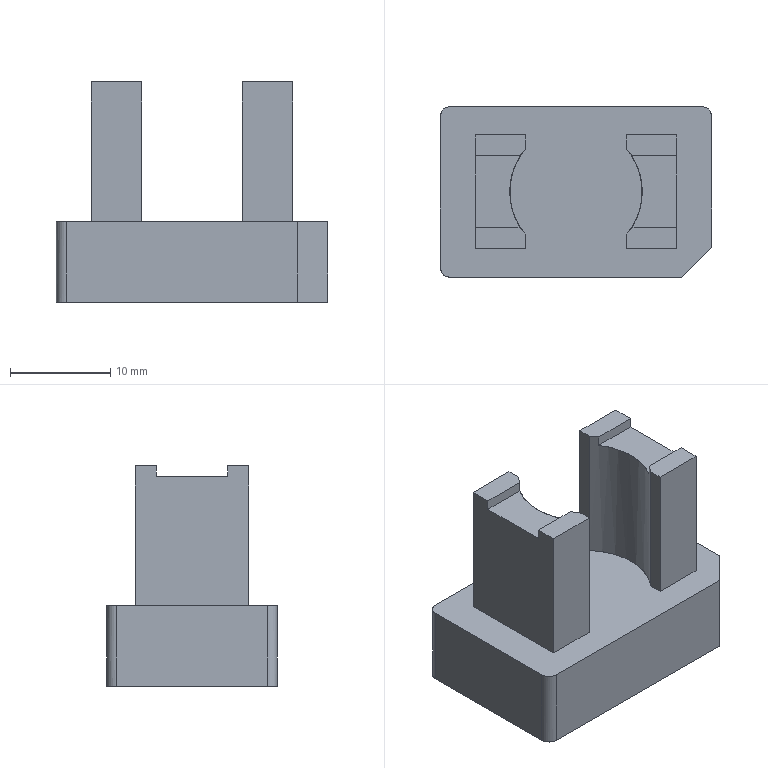NC program | PowerMill | posted with a generic post | part box 27 x 17 x 21.929 mm
Lines 5206 to 6181 of 116051:
N5303 M6
N5304 S18000 M03
N5305 G00 G90 X0.0 Y0.0
N5306 G43 Z9.7986 H2
N5307
N5308 G05 P10000 R4
N5309 X-12.0223 Y7.7454
N5310 Z0.7937
N5311 G01 Z-0.4063 F3600.0
N5312 X-11.8798 Y7.5778 F6000.0
N5313 X-11.4537 Y7.0768
N5314 X-11.2252 Y7.2711
N5315 X-10.7372 Y7.5319
N5316 X-10.2491 Y7.6444
N5317 X-4.8805 Y7.6519
N5318 X-4.3936 Y7.5648
N5319 X-3.9044 Y7.3367
N5320 X-3.5801 Y7.0768
N5321 X-3.4164 Y6.8936
N5322 X-3.218 Y6.5887
N5323 X-3.0368 Y6.1007
N5324 X-2.9865 Y5.6126
N5325 X-2.9947 Y4.1484
N5326 X-3.1019 Y3.6604
N5327 X-3.3555 Y3.1723
N5328 X-4.1012 Y2.1962
N5329 X-4.3925 Y1.9412
N5330 X-4.8182 Y1.7082
N5331 X-5.3686 Y1.5753
N5332 X-5.8566 Y1.5663
N5333 X-9.7611
N5334 X-10.2491 Y1.5765
N5335 X-10.7372 Y1.6889
N5336 X-11.2252 Y1.9498
N5337 X-11.5046 Y2.1962
N5338 X-11.7133 Y2.4594
N5339 X-11.8424 Y2.6843
N5340 X-12.0083 Y3.1723
N5341 X-12.0474 Y3.6604
N5342 Y5.6126
N5343 X-11.997 Y6.1007
N5344 X-11.816 Y6.5887
N5345 X-11.7133 Y6.7615
N5346 X-11.4537 Y7.0768
N5347 X-11.8798 Y7.5778
N5348 G00 Z3.7937
N5349 G01 X11.7989 Y7.9457 F10000.0
N5350 G00 Z0.7937
N5351 G01 Z-0.4063 F3600.0
N5352 X11.6564 Y7.7781 F6000.0
N5353 X11.2252 Y7.2711
N5354 X11.4537 Y7.0768
N5355 X11.7133 Y6.7615
N5356 X11.816 Y6.5887
N5357 X11.997 Y6.1007
N5358 X12.0474 Y5.6126
N5359 Y3.6604
N5360 X12.0083 Y3.1723
N5361 X11.8425 Y2.6843
N5362 X11.7133 Y2.4594
N5363 X11.5046 Y2.1962
N5364 X11.2252 Y1.9498
N5365 X10.7875 Y1.7082
N5366 X10.2491 Y1.5765
N5367 X9.7611 Y1.5663
N5368 X5.8566
N5369 X5.3686 Y1.5753
N5370 X4.8805 Y1.6846
N5371 X4.3925 Y1.9412
N5372 X4.1012 Y2.1962
N5373 X3.3555 Y3.1723
N5374 X3.1019 Y3.6604
N5375 X2.9947 Y4.1484
N5376 X2.9865 Y5.6126
N5377 X3.0368 Y6.1007
N5378 X3.218 Y6.5887
N5379 X3.4164 Y6.8936
N5380 X3.5801 Y7.0768
N5381 X3.9044 Y7.3367
N5382 X4.3925 Y7.5644
N5383 X4.8805 Y7.6519
N5384 X9.7611 Y7.6547
N5385 X10.2491 Y7.6444
N5386 X10.6403 Y7.5648
N5387 X11.2252 Y7.2711
N5388 X11.6564 Y7.7781
N5389 G00 Z3.7937
N5390 G01 X12.0223 Y-7.7454 F10000.0
N5391 G00 Z0.7937
N5392 G01 Z-0.4063 F3600.0
N5393 X11.8798 Y-7.5778 F6000.0
N5394 X11.4537 Y-7.0768
N5395 X11.2252 Y-7.2711
N5396 X10.6403 Y-7.5648
N5397 X10.2491 Y-7.6444
N5398 X4.8805 Y-7.6519
N5399 X4.3936 Y-7.5648
N5400 X3.9044 Y-7.3367
N5401 X3.5801 Y-7.0768
N5402 X3.4164 Y-6.8936
N5403 X3.218 Y-6.5887
N5404 X3.0368 Y-6.1007
N5405 X2.9865 Y-5.6126
N5406 X2.9947 Y-4.1484
N5407 X3.1019 Y-3.6604
N5408 X3.3555 Y-3.1723
N5409 X4.0954 Y-2.1962
N5410 X4.3925 Y-1.9302
N5411 X4.7819 Y-1.7082
N5412 X5.3686 Y-1.5561
N5413 X5.8566 Y-1.5458
N5414 X9.7611
N5415 X10.2491 Y-1.556
N5416 X10.7372 Y-1.6684
N5417 X11.2252 Y-1.9294
N5418 X11.5235 Y-2.1962
N5419 X11.7133 Y-2.4389
N5420 X11.8524 Y-2.6843
N5421 X12.0123 Y-3.1723
N5422 X12.0474 Y-3.6604
N5423 Y-5.6126
N5424 X11.997 Y-6.1007
N5425 X11.816 Y-6.5887
N5426 X11.7133 Y-6.7615
N5427 X11.4537 Y-7.0768
N5428 X11.8798 Y-7.5778
N5429 G00 Z3.7937
N5430 G01 X-11.7989 Y-7.9457 F10000.0
N5431 G00 Z0.7937
N5432 G01 Z-0.4063 F3600.0
N5433 X-11.6564 Y-7.7781 F6000.0
N5434 X-11.2252 Y-7.2711
N5435 X-11.4537 Y-7.0768
N5436 X-11.7133 Y-6.7615
N5437 X-11.816 Y-6.5887
N5438 X-11.997 Y-6.1007
N5439 X-12.0474 Y-5.6126
N5440 Y-3.6604
N5441 X-12.0122 Y-3.1723
N5442 X-11.8524 Y-2.6843
N5443 X-11.7133 Y-2.4389
N5444 X-11.5235 Y-2.1962
N5445 X-11.2252 Y-1.9294
N5446 X-10.8369 Y-1.7082
N5447 X-10.2491 Y-1.556
N5448 X-9.7611 Y-1.5458
N5449 X-5.8566
N5450 X-5.3686 Y-1.5561
N5451 X-4.8805 Y-1.6689
N5452 X-4.3925 Y-1.9302
N5453 X-4.0953 Y-2.1962
N5454 X-3.6415 Y-2.795
N5455 X-2.1015 Y-1.6849
N5456 X-0.5876 Y-0.5937
N5457 G03 X-0.1383 Y-0.87 I0.5563 J0.401
N5458 G03 X0.6469 Y-0.2942 I0.107 J0.6773
N5459 G01 X0.7056 Y0.0984
N5460 G03 X-0.6425 Y0.3114 I-0.675 J0.1009
N5461 G01 X-0.7077 Y-0.0801
N5462 G03 X-0.5876 Y-0.5937 I0.6764 J-0.1126
N5463 G01 X-2.1015 Y-1.6849
N5464 X-2.2353 Y-1.516
N5465 X-2.3761 Y-1.3529
N5466 X-2.7155 Y-0.9761
N5467 X-3.2416 Y-0.4349
N5468 G02 X-3.2218 Y0.4642 I0.4476 J0.4399
N5469 G01 X-2.7107 Y0.9402
N5470 G03 X-1.446 Y2.647 I-3.9757 J4.2682
N5471 G01 X-1.1868 Y3.1772
N5472 G02 X-0.4686 Y3.6259 I0.7188 J-0.3513
N5473 G01 X0.4658 Y3.6266
N5474 G02 X1.1573 Y3.2298 I0.0005 J-0.8
N5475 G01 X1.7618 Y2.1941
N5476 X2.0603 Y1.7401
N5477 X2.4055 Y1.3206
N5478 X2.7297 Y0.9668
N5479 X3.2386 Y0.4462
N5480 G02 X3.2213 Y-0.4564 I-0.4498 J-0.4428
N5481 G01 X2.7083 Y-0.939
N5482 G03 X1.3418 Y-2.8419 I4.1817 J-4.445
N5483 G01 X1.1966 Y-3.1588
N5484 G02 X0.4702 Y-3.6256 I-0.7273 J0.3332
N5485 G01 X-0.4653 Y-3.6267
N5486 G02 X-1.1572 Y-3.23 I-0.001 J0.8
N5487 G01 X-1.7618 Y-2.1941
N5488 X-1.924 Y-1.9344
N5489 X-2.1015 Y-1.6849
N5490 X-3.6415 Y-2.795
N5491 X-3.3555 Y-3.1723
N5492 X-3.1019 Y-3.6604
N5493 X-2.9947 Y-4.1484
N5494 X-2.9865 Y-5.6126
N5495 X-3.0368 Y-6.1007
N5496 X-3.218 Y-6.5887
N5497 X-3.4164 Y-6.8936
N5498 X-3.5801 Y-7.0768
N5499 X-3.9044 Y-7.3367
N5500 X-4.3936 Y-7.5648
N5501 X-4.8805 Y-7.6519
N5502 X-9.7611 Y-7.6547
N5503 X-10.2491 Y-7.6444
N5504 X-10.6403 Y-7.5648
N5505 X-11.2252 Y-7.2711
N5506 X-11.6564 Y-7.7781
N5507 G00 Z3.5984
N5508 G01 X-12.0223 Y7.7454 F10000.0
N5509 G00 Z0.5985
N5510 G01 Z-0.6015 F3600.0
N5511 X-11.8798 Y7.5778 F6000.0
N5512 X-11.4537 Y7.0768
N5513 X-11.2252 Y7.2711
N5514 X-10.7372 Y7.5319
N5515 X-10.2491 Y7.6444
N5516 X-4.8805 Y7.6519
N5517 X-4.3936 Y7.5648
N5518 X-3.9044 Y7.3367
N5519 X-3.5801 Y7.0768
N5520 X-3.4164 Y6.8936
N5521 X-3.218 Y6.5887
N5522 X-3.0368 Y6.1007
N5523 X-2.9865 Y5.6126
N5524 X-2.9947 Y4.1484
N5525 X-3.1019 Y3.6604
N5526 X-3.3555 Y3.1723
N5527 X-4.1012 Y2.1962
N5528 X-4.3925 Y1.9411
N5529 X-4.8182 Y1.7082
N5530 X-5.3686 Y1.5753
N5531 X-5.8566 Y1.5663
N5532 X-9.7611
N5533 X-10.2491 Y1.5764
N5534 X-10.7372 Y1.6889
N5535 X-11.2252 Y1.9497
N5536 X-11.5046 Y2.1962
N5537 X-11.7133 Y2.4593
N5538 X-11.8425 Y2.6843
N5539 X-12.0083 Y3.1723
N5540 X-12.0474 Y3.6604
N5541 Y5.6126
N5542 X-11.997 Y6.1007
N5543 X-11.816 Y6.5887
N5544 X-11.7133 Y6.7615
N5545 X-11.4537 Y7.0768
N5546 X-11.8798 Y7.5778
N5547 G00 Z3.5984
N5548 G01 X11.7989 Y7.9457 F10000.0
N5549 G00 Z0.5985
N5550 G01 Z-0.6015 F3600.0
N5551 X11.6564 Y7.7781 F6000.0
N5552 X11.2252 Y7.2711
N5553 X11.4537 Y7.0768
N5554 X11.7133 Y6.7615
N5555 X11.816 Y6.5887
N5556 X11.997 Y6.1007
N5557 X12.0474 Y5.6126
N5558 Y3.6604
N5559 X12.0083 Y3.1723
N5560 X11.8425 Y2.6843
N5561 X11.7133 Y2.4593
N5562 X11.5046 Y2.1962
N5563 X11.2252 Y1.9497
N5564 X10.7875 Y1.7082
N5565 X10.2491 Y1.5764
N5566 X9.7611 Y1.5663
N5567 X5.8566
N5568 X5.3686 Y1.5753
N5569 X4.8805 Y1.6846
N5570 X4.3925 Y1.9411
N5571 X4.1012 Y2.1962
N5572 X3.3555 Y3.1723
N5573 X3.1019 Y3.6604
N5574 X2.9947 Y4.1484
N5575 X2.9865 Y5.6126
N5576 X3.0368 Y6.1007
N5577 X3.218 Y6.5887
N5578 X3.4164 Y6.8936
N5579 X3.5801 Y7.0768
N5580 X3.9044 Y7.3367
N5581 X4.3925 Y7.5644
N5582 X4.8805 Y7.6519
N5583 X9.7611 Y7.6547
N5584 X10.2491 Y7.6444
N5585 X10.6403 Y7.5648
N5586 X11.2252 Y7.2711
N5587 X11.6564 Y7.7781
N5588 G00 Z3.5984
N5589 G01 X12.0223 Y-7.7454 F10000.0
N5590 G00 Z0.5985
N5591 G01 Z-0.6015 F3600.0
N5592 X11.8798 Y-7.5778 F6000.0
N5593 X11.4537 Y-7.0768
N5594 X11.2252 Y-7.2711
N5595 X10.6403 Y-7.5648
N5596 X10.2491 Y-7.6444
N5597 X4.8805 Y-7.6519
N5598 X4.3936 Y-7.5648
N5599 X3.9044 Y-7.3367
N5600 X3.5801 Y-7.0768
N5601 X3.4164 Y-6.8936
N5602 X3.218 Y-6.5887
N5603 X3.0368 Y-6.1007
N5604 X2.9865 Y-5.6126
N5605 X2.9947 Y-4.1484
N5606 X3.1019 Y-3.6604
N5607 X3.3555 Y-3.1723
N5608 X4.0954 Y-2.1962
N5609 X4.3925 Y-1.9302
N5610 X4.7819 Y-1.7082
N5611 X5.3686 Y-1.5561
N5612 X5.8566 Y-1.5458
N5613 X9.7611
N5614 X10.2491 Y-1.556
N5615 X10.7372 Y-1.6684
N5616 X11.2252 Y-1.9294
N5617 X11.5235 Y-2.1962
N5618 X11.7133 Y-2.4389
N5619 X11.8525 Y-2.6843
N5620 X12.0123 Y-3.1723
N5621 X12.0474 Y-3.6604
N5622 Y-5.6126
N5623 X11.997 Y-6.1007
N5624 X11.816 Y-6.5887
N5625 X11.7133 Y-6.7615
N5626 X11.4537 Y-7.0768
N5627 X11.8798 Y-7.5778
N5628 G00 Z3.5984
N5629 G01 X-11.7989 Y-7.9457 F10000.0
N5630 G00 Z0.5985
N5631 G01 Z-0.6015 F3600.0
N5632 X-11.6564 Y-7.7781 F6000.0
N5633 X-11.2252 Y-7.2711
N5634 X-11.4537 Y-7.0768
N5635 X-11.7133 Y-6.7615
N5636 X-11.816 Y-6.5887
N5637 X-11.997 Y-6.1007
N5638 X-12.0474 Y-5.6126
N5639 Y-3.6604
N5640 X-12.0123 Y-3.1723
N5641 X-11.8524 Y-2.6843
N5642 X-11.7133 Y-2.4389
N5643 X-11.5235 Y-2.1962
N5644 X-11.2252 Y-1.9294
N5645 X-10.8369 Y-1.7082
N5646 X-10.2491 Y-1.556
N5647 X-9.7611 Y-1.5458
N5648 X-5.8566
N5649 X-5.3686 Y-1.5561
N5650 X-4.8805 Y-1.6689
N5651 X-4.3925 Y-1.9302
N5652 X-4.0953 Y-2.1962
N5653 X-3.6412 Y-2.7954
N5654 X-2.1013 Y-1.6852
N5655 X-0.5875 Y-0.5938
N5656 G03 X-0.1382 Y-0.8701 I0.5562 J0.401
N5657 G03 X0.6469 Y-0.2941 I0.1069 J0.6773
N5658 G01 X0.7056 Y0.0985
N5659 G03 X-0.6425 Y0.3114 I-0.675 J0.1009
N5660 G01 X-0.7077 Y-0.0802
N5661 G03 X-0.5875 Y-0.5938 I0.6764 J-0.1126
N5662 G01 X-2.1013 Y-1.6852
N5663 X-2.2352 Y-1.5162
N5664 X-2.376 Y-1.353
N5665 X-2.7155 Y-0.9761
N5666 X-3.2416 Y-0.4349
N5667 G02 X-3.2217 Y0.4642 I0.4476 J0.4399
N5668 G01 X-2.7107 Y0.9402
N5669 G03 X-1.4467 Y2.6458 I-3.9752 J4.2674
N5670 G01 X-1.1867 Y3.1774
N5671 G02 X-0.4686 Y3.6259 I0.7187 J-0.3515
N5672 G01 X0.4658 Y3.6266
N5673 G02 X1.1573 Y3.2298 I0.0005 J-0.8
N5674 G01 X1.7618 Y2.1941
N5675 X2.0602 Y1.7402
N5676 X2.4054 Y1.3207
N5677 X2.7297 Y0.9668
N5678 X3.2386 Y0.4462
N5679 G02 X3.2213 Y-0.4564 I-0.4499 J-0.4428
N5680 G01 X2.7083 Y-0.939
N5681 G03 X1.3426 Y-2.8402 I4.1812 J-4.4444
N5682 G01 X1.1965 Y-3.159
N5683 G02 X0.4702 Y-3.6256 I-0.7272 J0.3334
N5684 G01 X-0.4653 Y-3.6267
N5685 G02 X-1.1572 Y-3.23 I-0.001 J0.8
N5686 G01 X-1.7618 Y-2.1941
N5687 X-1.9239 Y-1.9345
N5688 X-2.1013 Y-1.6852
N5689 X-3.6412 Y-2.7954
N5690 X-3.3555 Y-3.1723
N5691 X-3.1019 Y-3.6604
N5692 X-2.9947 Y-4.1484
N5693 X-2.9865 Y-5.6126
N5694 X-3.0368 Y-6.1007
N5695 X-3.218 Y-6.5887
N5696 X-3.4164 Y-6.8936
N5697 X-3.5801 Y-7.0768
N5698 X-3.9044 Y-7.3367
N5699 X-4.3936 Y-7.5648
N5700 X-4.8805 Y-7.6519
N5701 X-9.7611 Y-7.6547
N5702 X-10.2491 Y-7.6444
N5703 X-10.6403 Y-7.5648
N5704 X-11.2252 Y-7.2711
N5705 X-11.6564 Y-7.7781
N5706 G00 Z3.4032
N5707 G01 X-12.0223 Y7.7454 F10000.0
N5708 G00 Z0.4032
N5709 G01 Z-0.7968 F3600.0
N5710 X-11.8798 Y7.5778 F6000.0
N5711 X-11.4537 Y7.0768
N5712 X-11.2252 Y7.2711
N5713 X-10.7372 Y7.5319
N5714 X-10.2491 Y7.6444
N5715 X-4.8805 Y7.6519
N5716 X-4.3936 Y7.5648
N5717 X-3.9044 Y7.3367
N5718 X-3.5801 Y7.0768
N5719 X-3.4164 Y6.8936
N5720 X-3.218 Y6.5887
N5721 X-3.0368 Y6.1007
N5722 X-2.9865 Y5.6126
N5723 X-2.9947 Y4.1484
N5724 X-3.1018 Y3.6604
N5725 X-3.3555 Y3.1723
N5726 X-4.1012 Y2.1962
N5727 X-4.3925 Y1.9411
N5728 X-4.8182 Y1.7082
N5729 X-5.3686 Y1.5753
N5730 X-5.8566 Y1.5662
N5731 X-9.7611
N5732 X-10.2491 Y1.5764
N5733 X-10.7372 Y1.6889
N5734 X-11.2252 Y1.9497
N5735 X-11.5046 Y2.1962
N5736 X-11.7133 Y2.4593
N5737 X-11.8425 Y2.6843
N5738 X-12.0084 Y3.1723
N5739 X-12.0474 Y3.6604
N5740 Y5.6126
N5741 X-11.997 Y6.1007
N5742 X-11.816 Y6.5887
N5743 X-11.7133 Y6.7615
N5744 X-11.4537 Y7.0768
N5745 X-11.8798 Y7.5778
N5746 G00 Z3.4032
N5747 G01 X11.7989 Y7.9457 F10000.0
N5748 G00 Z0.4032
N5749 G01 Z-0.7968 F3600.0
N5750 X11.6564 Y7.7781 F6000.0
N5751 X11.2252 Y7.2711
N5752 X11.4537 Y7.0768
N5753 X11.7133 Y6.7615
N5754 X11.816 Y6.5887
N5755 X11.997 Y6.1007
N5756 X12.0474 Y5.6126
N5757 Y3.6604
N5758 X12.0083 Y3.1723
N5759 X11.8425 Y2.6843
N5760 X11.7133 Y2.4593
N5761 X11.5046 Y2.1962
N5762 X11.2252 Y1.9497
N5763 X10.7875 Y1.7082
N5764 X10.2491 Y1.5764
N5765 X9.7611 Y1.5662
N5766 X5.8566
N5767 X5.3686 Y1.5753
N5768 X4.8805 Y1.6845
N5769 X4.3925 Y1.9411
N5770 X4.1012 Y2.1962
N5771 X3.3555 Y3.1723
N5772 X3.1018 Y3.6604
N5773 X2.9947 Y4.1484
N5774 X2.9865 Y5.6126
N5775 X3.0368 Y6.1007
N5776 X3.218 Y6.5887
N5777 X3.4164 Y6.8936
N5778 X3.5801 Y7.0768
N5779 X3.9044 Y7.3367
N5780 X4.3925 Y7.5644
N5781 X4.8805 Y7.6519
N5782 X9.7611 Y7.6547
N5783 X10.2491 Y7.6444
N5784 X10.6403 Y7.5648
N5785 X11.2252 Y7.2711
N5786 X11.6564 Y7.7781
N5787 G00 Z3.4032
N5788 G01 X12.0223 Y-7.7454 F10000.0
N5789 G00 Z0.4032
N5790 G01 Z-0.7968 F3600.0
N5791 X11.8798 Y-7.5778 F6000.0
N5792 X11.4537 Y-7.0768
N5793 X11.2252 Y-7.2711
N5794 X10.6403 Y-7.5648
N5795 X10.2491 Y-7.6444
N5796 X4.8805 Y-7.6519
N5797 X4.3936 Y-7.5648
N5798 X3.9044 Y-7.3367
N5799 X3.5801 Y-7.0768
N5800 X3.4164 Y-6.8936
N5801 X3.218 Y-6.5887
N5802 X3.0368 Y-6.1007
N5803 X2.9865 Y-5.6126
N5804 X2.9947 Y-4.1484
N5805 X3.1018 Y-3.6604
N5806 X3.3555 Y-3.1723
N5807 X4.0953 Y-2.1962
N5808 X4.3925 Y-1.9301
N5809 X4.7819 Y-1.7082
N5810 X5.3686 Y-1.5561
N5811 X5.8566 Y-1.5458
N5812 X9.7611
N5813 X10.2491 Y-1.556
N5814 X10.7372 Y-1.6684
N5815 X11.2252 Y-1.9293
N5816 X11.5236 Y-2.1962
N5817 X11.7133 Y-2.4389
N5818 X11.8525 Y-2.6843
N5819 X12.0123 Y-3.1723
N5820 X12.0474 Y-3.6604
N5821 Y-5.6126
N5822 X11.997 Y-6.1007
N5823 X11.816 Y-6.5887
N5824 X11.7133 Y-6.7615
N5825 X11.4537 Y-7.0768
N5826 X11.8798 Y-7.5778
N5827 G00 Z3.4032
N5828 G01 X-11.7989 Y-7.9457 F10000.0
N5829 G00 Z0.4032
N5830 G01 Z-0.7968 F3600.0
N5831 X-11.6564 Y-7.7781 F6000.0
N5832 X-11.2252 Y-7.2711
N5833 X-11.4537 Y-7.0768
N5834 X-11.7133 Y-6.7615
N5835 X-11.816 Y-6.5887
N5836 X-11.997 Y-6.1007
N5837 X-12.0474 Y-5.6126
N5838 Y-3.6604
N5839 X-12.0123 Y-3.1723
N5840 X-11.8524 Y-2.6843
N5841 X-11.7133 Y-2.4389
N5842 X-11.5235 Y-2.1962
N5843 X-11.2252 Y-1.9293
N5844 X-10.837 Y-1.7082
N5845 X-10.2491 Y-1.556
N5846 X-9.7611 Y-1.5458
N5847 X-5.8566
N5848 X-5.3686 Y-1.5561
N5849 X-4.8805 Y-1.6689
N5850 X-4.3925 Y-1.9301
N5851 X-4.0953 Y-2.1962
N5852 X-3.6416 Y-2.7949
N5853 X-2.1016 Y-1.6849
N5854 X-0.5876 Y-0.5937
N5855 G03 X-0.1383 Y-0.87 I0.5563 J0.401
N5856 G03 X0.6469 Y-0.294 I0.107 J0.6773
N5857 G01 X0.7055 Y0.0987
N5858 G03 X-0.6425 Y0.3116 I-0.6749 J0.1008
N5859 G01 X-0.7077 Y-0.08
N5860 G03 X-0.5876 Y-0.5937 I0.6764 J-0.1127
N5861 G01 X-2.1016 Y-1.6849
N5862 X-2.237 Y-1.514
N5863 X-2.3796 Y-1.349
N5864 X-2.774 Y-0.9122
N5865 X-3.242 Y-0.428
N5866 G02 X-3.2202 Y0.4656 I0.4481 J0.4361
N5867 G01 X-2.7105 Y0.9404
N5868 G03 X-1.4474 Y2.6446 I-3.9749 J4.2665
N5869 G01 X-1.1867 Y3.1775
N5870 G02 X-0.4686 Y3.6259 I0.7187 J-0.3516
N5871 G01 X0.4658 Y3.6266
N5872 G02 X1.1573 Y3.2299 I0.0005 J-0.8
N5873 G01 X1.7618 Y2.1941
N5874 X2.0602 Y1.7403
N5875 X2.4053 Y1.3208
N5876 X2.7297 Y0.9668
N5877 X3.2386 Y0.4462
N5878 G02 X3.2212 Y-0.4564 I-0.4499 J-0.4428
N5879 G01 X2.7082 Y-0.939
N5880 G03 X1.3489 Y-2.8265 I4.1813 J-4.4445
N5881 G01 X1.1944 Y-3.1613
N5882 G02 X0.4685 Y-3.6261 I-0.7264 J0.3352
N5883 G01 X-0.4657 Y-3.6267
N5884 G02 X-1.1572 Y-3.23 I-0.0006 J0.8
N5885 G01 X-1.7618 Y-2.1941
N5886 X-1.924 Y-1.9344
N5887 X-2.1016 Y-1.6849
N5888 X-3.6416 Y-2.7949
N5889 X-3.3555 Y-3.1723
N5890 X-3.1018 Y-3.6604
N5891 X-2.9947 Y-4.1484
N5892 X-2.9865 Y-5.6126
N5893 X-3.0368 Y-6.1007
N5894 X-3.218 Y-6.5887
N5895 X-3.4164 Y-6.8936
N5896 X-3.5801 Y-7.0768
N5897 X-3.9044 Y-7.3367
N5898 X-4.3936 Y-7.5648
N5899 X-4.8805 Y-7.6519
N5900 X-9.7611 Y-7.6547
N5901 X-10.2491 Y-7.6444
N5902 X-10.6403 Y-7.5648
N5903 X-11.2252 Y-7.2711
N5904 X-11.6564 Y-7.7781
N5905 G00 Z3.2079
N5906 G01 X-12.0223 Y7.7454 F10000.0
N5907 G00 Z0.2079
N5908 G01 Z-0.9921 F3600.0
N5909 X-11.8798 Y7.5778 F6000.0
N5910 X-11.4537 Y7.0768
N5911 X-11.2252 Y7.2711
N5912 X-10.7372 Y7.5319
N5913 X-10.2491 Y7.6444
N5914 X-4.8805 Y7.6519
N5915 X-4.3936 Y7.5648
N5916 X-3.9044 Y7.3367
N5917 X-3.5801 Y7.0768
N5918 X-3.4164 Y6.8936
N5919 X-3.218 Y6.5887
N5920 X-3.0368 Y6.1007
N5921 X-2.9865 Y5.6126
N5922 X-2.9947 Y4.1484
N5923 X-3.1018 Y3.6604
N5924 X-3.3555 Y3.1723
N5925 X-4.1012 Y2.1962
N5926 X-4.3925 Y1.9411
N5927 X-4.8182 Y1.7082
N5928 X-5.3686 Y1.5753
N5929 X-5.8566 Y1.5662
N5930 X-9.7611
N5931 X-10.2491 Y1.5764
N5932 X-10.7372 Y1.6889
N5933 X-11.2252 Y1.9497
N5934 X-11.5046 Y2.1962
N5935 X-11.7133 Y2.4593
N5936 X-11.8425 Y2.6843
N5937 X-12.0084 Y3.1723
N5938 X-12.0474 Y3.6604
N5939 Y5.6126
N5940 X-11.997 Y6.1007
N5941 X-11.816 Y6.5887
N5942 X-11.7133 Y6.7615
N5943 X-11.4537 Y7.0768
N5944 X-11.8798 Y7.5778
N5945 G00 Z3.2079
N5946 G01 X11.7989 Y7.9457 F10000.0
N5947 G00 Z0.2079
N5948 G01 Z-0.9921 F3600.0
N5949 X11.6564 Y7.7781 F6000.0
N5950 X11.2252 Y7.2711
N5951 X11.4537 Y7.0768
N5952 X11.7133 Y6.7615
N5953 X11.816 Y6.5887
N5954 X11.997 Y6.1007
N5955 X12.0474 Y5.6126
N5956 Y3.6604
N5957 X12.0083 Y3.1723
N5958 X11.8426 Y2.6843
N5959 X11.7133 Y2.4593
N5960 X11.5046 Y2.1962
N5961 X11.2252 Y1.9497
N5962 X10.7875 Y1.7082
N5963 X10.2491 Y1.5764
N5964 X9.7611 Y1.5662
N5965 X5.8566
N5966 X5.3686 Y1.5753
N5967 X4.8805 Y1.6845
N5968 X4.3925 Y1.9411
N5969 X4.1011 Y2.1962
N5970 X3.3555 Y3.1723
N5971 X3.1018 Y3.6604
N5972 X2.9947 Y4.1484
N5973 X2.9865 Y5.6126
N5974 X3.0368 Y6.1007
N5975 X3.218 Y6.5887
N5976 X3.4164 Y6.8936
N5977 X3.5801 Y7.0768
N5978 X3.9044 Y7.3367
N5979 X4.3925 Y7.5644
N5980 X4.8805 Y7.6519
N5981 X9.7611 Y7.6547
N5982 X10.2491 Y7.6444
N5983 X10.6403 Y7.5648
N5984 X11.2252 Y7.2711
N5985 X11.6564 Y7.7781
N5986 G00 Z3.2079
N5987 G01 X12.0223 Y-7.7454 F10000.0
N5988 G00 Z0.2079
N5989 G01 Z-0.9921 F3600.0
N5990 X11.8798 Y-7.5778 F6000.0
N5991 X11.4537 Y-7.0768
N5992 X11.2252 Y-7.2711
N5993 X10.6403 Y-7.5648
N5994 X10.2491 Y-7.6444
N5995 X4.8805 Y-7.6519
N5996 X4.3936 Y-7.5648
N5997 X3.9044 Y-7.3367
N5998 X3.5801 Y-7.0768
N5999 X3.4164 Y-6.8936
N6000 X3.218 Y-6.5887
N6001 X3.0368 Y-6.1007
N6002 X2.9865 Y-5.6126
N6003 X2.9947 Y-4.1484
N6004 X3.1018 Y-3.6604
N6005 X3.3555 Y-3.1723
N6006 X4.0953 Y-2.1962
N6007 X4.3925 Y-1.9301
N6008 X4.7818 Y-1.7082
N6009 X5.3686 Y-1.5561
N6010 X5.8566 Y-1.5458
N6011 X9.7611
N6012 X10.2491 Y-1.5559
N6013 X10.7372 Y-1.6684
N6014 X11.2252 Y-1.9293
N6015 X11.5236 Y-2.1962
N6016 X11.7133 Y-2.4389
N6017 X11.8525 Y-2.6843
N6018 X12.0123 Y-3.1723
N6019 X12.0474 Y-3.6604
N6020 Y-5.6126
N6021 X11.997 Y-6.1007
N6022 X11.816 Y-6.5887
N6023 X11.7133 Y-6.7615
N6024 X11.4537 Y-7.0768
N6025 X11.8798 Y-7.5778
N6026 G00 Z3.2079
N6027 G01 X-11.7989 Y-7.9457 F10000.0
N6028 G00 Z0.2079
N6029 G01 Z-0.9921 F3600.0
N6030 X-11.6564 Y-7.7781 F6000.0
N6031 X-11.2252 Y-7.2711
N6032 X-11.4537 Y-7.0768
N6033 X-11.7133 Y-6.7615
N6034 X-11.816 Y-6.5887
N6035 X-11.997 Y-6.1007
N6036 X-12.0474 Y-5.6126
N6037 Y-3.6604
N6038 X-12.0123 Y-3.1723
N6039 X-11.8524 Y-2.6843
N6040 X-11.7133 Y-2.4389
N6041 X-11.5236 Y-2.1962
N6042 X-11.2252 Y-1.9293
N6043 X-10.837 Y-1.7082
N6044 X-10.2491 Y-1.5559
N6045 X-9.7611 Y-1.5458
N6046 X-5.8566
N6047 X-5.3686 Y-1.5561
N6048 X-4.8805 Y-1.6689
N6049 X-4.3925 Y-1.9301
N6050 X-4.0953 Y-2.1962
N6051 X-3.6413 Y-2.7953
N6052 X-2.1014 Y-1.6851
N6053 X-0.5875 Y-0.5938
N6054 G03 X-0.1382 Y-0.8701 I0.5562 J0.401
N6055 G03 X0.6469 Y-0.294 I0.1069 J0.6773
N6056 G01 X0.7055 Y0.0988
N6057 G03 X-0.6425 Y0.3116 I-0.6749 J0.1007
N6058 G01 X-0.7077 Y-0.0801
N6059 G03 X-0.5875 Y-0.5938 I0.6764 J-0.1127
N6060 G01 X-2.1014 Y-1.6851
N6061 X-2.2369 Y-1.5141
N6062 X-2.3796 Y-1.3491
N6063 X-2.7739 Y-0.9122
N6064 X-3.242 Y-0.428
N6065 G02 X-3.2016 Y0.4821 I0.4481 J0.4361
N6066 G01 X-3.0472 Y0.615
N6067 X-2.8389 Y0.803
N6068 X-2.6399 Y1.0007
N6069 X-2.4775 Y1.1701
N6070 G03 X-1.4481 Y2.6433 I-4.2074 J4.036
N6071 G01 X-1.1866 Y3.1776
N6072 G02 X-0.4686 Y3.6259 I0.7186 J-0.3517
N6073 G01 X0.4658 Y3.6265
N6074 G02 X1.1573 Y3.2298 I0.0006 J-0.8
N6075 G01 X1.7618 Y2.194
N6076 X2.0602 Y1.7403
N6077 X2.4051 Y1.321
N6078 X2.7296 Y0.9669
N6079 X3.2385 Y0.4462
N6080 G02 X3.2212 Y-0.4564 I-0.4498 J-0.4428
N6081 G01 X2.7082 Y-0.939
N6082 G03 X1.3497 Y-2.8249 I4.1808 J-4.4438
N6083 G01 X1.1943 Y-3.1615
N6084 G02 X0.4685 Y-3.6261 I-0.7263 J0.3354
N6085 G01 X-0.4657 Y-3.6267
N6086 G02 X-1.1572 Y-3.23 I-0.0006 J0.8
N6087 G01 X-1.7618 Y-2.1941
N6088 X-1.9239 Y-1.9345
N6089 X-2.1014 Y-1.6851
N6090 X-3.6413 Y-2.7953
N6091 X-3.3555 Y-3.1723
N6092 X-3.1018 Y-3.6604
N6093 X-2.9947 Y-4.1484
N6094 X-2.9865 Y-5.6126
N6095 X-3.0368 Y-6.1007
N6096 X-3.218 Y-6.5887
N6097 X-3.4164 Y-6.8936
N6098 X-3.5801 Y-7.0768
N6099 X-3.9044 Y-7.3367
N6100 X-4.3936 Y-7.5648
N6101 X-4.8805 Y-7.6519
N6102 X-9.7611 Y-7.6547
N6103 X-10.2491 Y-7.6444
N6104 X-10.6403 Y-7.5648
N6105 X-11.2252 Y-7.2711
N6106 X-11.6564 Y-7.7781
N6107 G00 Z3.0126
N6108 G01 X-12.0223 Y7.7454 F10000.0
N6109 G00 Z0.0126
N6110 G01 Z-1.1874 F3600.0
N6111 X-11.8798 Y7.5778 F6000.0
N6112 X-11.4537 Y7.0768
N6113 X-11.2252 Y7.2711
N6114 X-10.7372 Y7.5319
N6115 X-10.2491 Y7.6444
N6116 X-4.8805 Y7.6519
N6117 X-4.3936 Y7.5648
N6118 X-3.9044 Y7.3367
N6119 X-3.5801 Y7.0768
N6120 X-3.4164 Y6.8936
N6121 X-3.218 Y6.5887
N6122 X-3.0368 Y6.1007
N6123 X-2.9865 Y5.6126
N6124 X-2.9947 Y4.1484
N6125 X-3.1018 Y3.6604
N6126 X-3.3555 Y3.1723
N6127 X-4.1012 Y2.1962
N6128 X-4.3925 Y1.9411
N6129 X-4.8181 Y1.7082
N6130 X-5.3686 Y1.5752
N6131 X-5.8566 Y1.5662
N6132 X-9.7611
N6133 X-10.2491 Y1.5764
N6134 X-10.7372 Y1.6889
N6135 X-11.2252 Y1.9497
N6136 X-11.5046 Y2.1962
N6137 X-11.7133 Y2.4593
N6138 X-11.8425 Y2.6843
N6139 X-12.0084 Y3.1723
N6140 X-12.0474 Y3.6604
N6141 Y5.6126
N6142 X-11.997 Y6.1007
N6143 X-11.816 Y6.5887
N6144 X-11.7133 Y6.7615
N6145 X-11.4537 Y7.0768
N6146 X-11.8798 Y7.5778
N6147 G00 Z3.0126
N6148 G01 X11.7989 Y7.9457 F10000.0
N6149 G00 Z0.0126
N6150 G01 Z-1.1874 F3600.0
N6151 X11.6564 Y7.7781 F6000.0
N6152 X11.2252 Y7.2711
N6153 X11.4537 Y7.0768
N6154 X11.7133 Y6.7615
N6155 X11.816 Y6.5887
N6156 X11.997 Y6.1007
N6157 X12.0474 Y5.6126
N6158 Y3.6604
N6159 X12.0084 Y3.1723
N6160 X11.8426 Y2.6843
N6161 X11.7133 Y2.4593
N6162 X11.5046 Y2.1962
N6163 X11.2252 Y1.9497
N6164 X10.7875 Y1.7082
N6165 X10.2491 Y1.5764
N6166 X9.7611 Y1.5662
N6167 X5.8566
N6168 X5.3686 Y1.5752
N6169 X4.8805 Y1.6845
N6170 X4.3925 Y1.9411
N6171 X4.1011 Y2.1962
N6172 X3.3555 Y3.1723
N6173 X3.1018 Y3.6604
N6174 X2.9947 Y4.1484
N6175 X2.9865 Y5.6126
N6176 X3.0368 Y6.1007
N6177 X3.218 Y6.5887
N6178 X3.4164 Y6.8936
N6179 X3.5801 Y7.0768
N6180 X3.9044 Y7.3367
N6181 X4.3925 Y7.5644
N6182 X4.8805 Y7.6519
N6183 X9.7611 Y7.6547
N6184 X10.2491 Y7.6444
N6185 X10.6403 Y7.5648
N6186 X11.2252 Y7.2711
N6187 X11.6564 Y7.7781
N6188 G00 Z3.0126
N6189 G01 X12.0223 Y-7.7454 F10000.0
N6190 G00 Z0.0126
N6191 G01 Z-1.1874 F3600.0
N6192 X11.8798 Y-7.5778 F6000.0
N6193 X11.4537 Y-7.0768
N6194 X11.2252 Y-7.2711
N6195 X10.6403 Y-7.5648
N6196 X10.2491 Y-7.6444
N6197 X4.8805 Y-7.6519
N6198 X4.3936 Y-7.5648
N6199 X3.9044 Y-7.3367
N6200 X3.5801 Y-7.0768
N6201 X3.4164 Y-6.8936
N6202 X3.218 Y-6.5887
N6203 X3.0368 Y-6.1007
N6204 X2.9865 Y-5.6126
N6205 X2.9947 Y-4.1484
N6206 X3.1018 Y-3.6604
N6207 X3.3555 Y-3.1723
N6208 X4.0953 Y-2.1962
N6209 X4.3925 Y-1.9301
N6210 X4.7818 Y-1.7082
N6211 X5.3686 Y-1.556
N6212 X5.8566 Y-1.5457
N6213 X9.7611
N6214 X10.2491 Y-1.5559
N6215 X10.7372 Y-1.6684
N6216 X11.2252 Y-1.9293
N6217 X11.5236 Y-2.1962
N6218 X11.7133 Y-2.4388
N6219 X11.8525 Y-2.6843
N6220 X12.0124 Y-3.1723
N6221 X12.0474 Y-3.6604
N6222 Y-5.6126
N6223 X11.997 Y-6.1007
N6224 X11.816 Y-6.5887
N6225 X11.7133 Y-6.7615
N6226 X11.4537 Y-7.0768
N6227 X11.8798 Y-7.5778
N6228 G00 Z3.0126
N6229 G01 X-11.7989 Y-7.9457 F10000.0
N6230 G00 Z0.0126
N6231 G01 Z-1.1874 F3600.0
N6232 X-11.6564 Y-7.7781 F6000.0
N6233 X-11.2252 Y-7.2711
N6234 X-11.4537 Y-7.0768
N6235 X-11.7133 Y-6.7615
N6236 X-11.816 Y-6.5887
N6237 X-11.997 Y-6.1007
N6238 X-12.0474 Y-5.6126
N6239 Y-3.6604
N6240 X-12.0123 Y-3.1723
N6241 X-11.8525 Y-2.6843
N6242 X-11.7133 Y-2.4388
N6243 X-11.5236 Y-2.1962
N6244 X-11.2252 Y-1.9293
N6245 X-10.837 Y-1.7082
N6246 X-10.2491 Y-1.5559
N6247 X-9.7611 Y-1.5457
N6248 X-5.8566
N6249 X-5.3686 Y-1.556
N6250 X-4.8805 Y-1.6688
N6251 X-4.3925 Y-1.9301
N6252 X-4.0953 Y-2.1962
N6253 X-3.6403 Y-2.7966
N6254 X-2.1008 Y-1.686
N6255 X-0.5873 Y-0.5941
N6256 G03 X-0.138 Y-0.8702 I0.556 J0.4012
N6257 G03 X0.6469 Y-0.294 I0.1067 J0.6773
N6258 G01 X0.7054 Y0.099
N6259 G03 X-0.6425 Y0.3114 I-0.6748 J0.1006
N6260 G01 X-0.7076 Y-0.0806
N6261 G03 X-0.5873 Y-0.5941 I0.6763 J-0.1123
N6262 G01 X-2.1008 Y-1.686
N6263 X-2.2347 Y-1.5167
N6264 X-2.3758 Y-1.3533
N6265 X-2.7153 Y-0.9762
N6266 X-3.2415 Y-0.4349
N6267 G02 X-3.2217 Y0.4642 I0.4476 J0.4399
N6268 G01 X-2.7107 Y0.9402
N6269 G03 X-1.4488 Y2.642 I-3.9736 J4.2652
N6270 G01 X-1.1866 Y3.1777
N6271 G02 X-0.4686 Y3.6259 I0.7186 J-0.3518
N6272 G01 X0.4658 Y3.6265
N6273 G02 X1.1573 Y3.2298 I0.0006 J-0.8
N6274 G01 X1.7618 Y2.194
N6275 X2.0601 Y1.7404
N6276 X2.405 Y1.3211
N6277 X2.7296 Y0.9669
N6278 X3.2385 Y0.4462